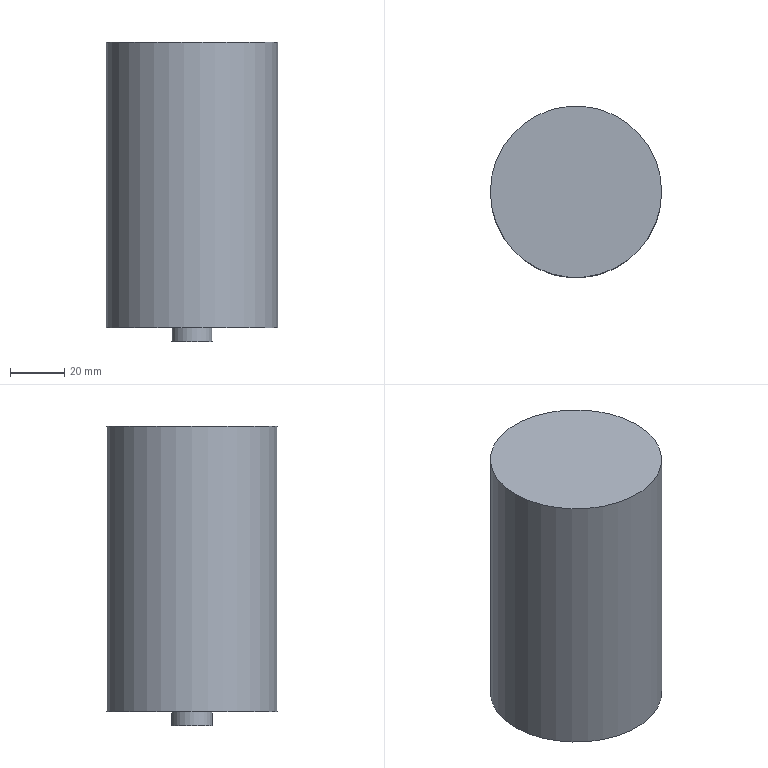Part | NX | features solid 2 | 1 solid | 5 faces | box 63 x 63 x 110 mm | volume 328194 mm3 | plane 3 | cylinder 2 | commonest cylinder face diameters 15 x1 63 x1
STEP:
#1=CARTESIAN_POINT('',(1245.,-607.5,-145.));
#2=VERTEX_POINT('',#1);
#3=CARTESIAN_POINT('',(1245.,-615.,-145.));
#4=DIRECTION('',(0.,0.,1.));
#5=DIRECTION('',(0.,1.,0.));
#6=AXIS2_PLACEMENT_3D('',#3,#4,#5);
#7=CIRCLE('',#6,7.5);
#8=EDGE_CURVE('',#2,#2,#7,.T.);
#9=ORIENTED_EDGE('',*,*,#8,.F.);
#10=EDGE_LOOP('',(#9));
#11=FACE_BOUND('',#10,.T.);
#12=CARTESIAN_POINT('',(1245.,-615.,-145.));
#13=DIRECTION('',(0.,0.,-1.));
#14=DIRECTION('',(0.,-1.,0.));
#15=AXIS2_PLACEMENT_3D('',#12,#13,#14);
#16=PLANE('',#15);
#17=ADVANCED_FACE('',(#11),#16,.T.);
#18=CARTESIAN_POINT('',(1245.,-607.5,-140.));
#19=VERTEX_POINT('',#18);
#20=CARTESIAN_POINT('',(1245.,-615.,-140.));
#21=DIRECTION('',(0.,0.,1.));
#22=DIRECTION('',(0.,1.,0.));
#23=AXIS2_PLACEMENT_3D('',#20,#21,#22);
#24=CIRCLE('',#23,7.5);
#25=EDGE_CURVE('',#19,#19,#24,.T.);
#26=ORIENTED_EDGE('',*,*,#25,.F.);
#27=EDGE_LOOP('',(#26));
#28=FACE_BOUND('',#27,.T.);
#29=ORIENTED_EDGE('',*,*,#8,.T.);
#30=EDGE_LOOP('',(#29));
#31=FACE_BOUND('',#30,.T.);
#32=CARTESIAN_POINT('',(1245.,-615.,-140.));
#33=DIRECTION('',(0.,0.,1.));
#34=DIRECTION('',(0.,1.,0.));
#35=AXIS2_PLACEMENT_3D('',#32,#33,#34);
#36=CYLINDRICAL_SURFACE('',#35,7.5);
#37=ADVANCED_FACE('',(#28,#31),#36,.T.);
#38=CARTESIAN_POINT('',(1213.5,-615.,-35.));
#39=VERTEX_POINT('',#38);
#40=CARTESIAN_POINT('',(1245.,-615.,-35.));
#41=DIRECTION('',(0.,0.,-1.));
#42=DIRECTION('',(-1.,0.,0.));
#43=AXIS2_PLACEMENT_3D('',#40,#41,#42);
#44=CIRCLE('',#43,31.5);
#45=EDGE_CURVE('',#39,#39,#44,.T.);
#46=ORIENTED_EDGE('',*,*,#45,.F.);
#47=EDGE_LOOP('',(#46));
#48=FACE_BOUND('',#47,.T.);
#49=CARTESIAN_POINT('',(1250.,-750.,-35.));
#50=DIRECTION('',(0.,0.,1.));
#51=DIRECTION('',(0.,-1.,0.));
#52=AXIS2_PLACEMENT_3D('',#49,#50,#51);
#53=PLANE('',#52);
#54=ADVANCED_FACE('',(#48),#53,.T.);
#55=ORIENTED_EDGE('',*,*,#25,.T.);
#56=EDGE_LOOP('',(#55));
#57=FACE_BOUND('',#56,.T.);
#58=CARTESIAN_POINT('',(1276.5,-615.,-140.));
#59=VERTEX_POINT('',#58);
#60=CARTESIAN_POINT('',(1245.,-615.,-140.));
#61=DIRECTION('',(0.,0.,1.));
#62=DIRECTION('',(1.,0.,0.));
#63=AXIS2_PLACEMENT_3D('',#60,#61,#62);
#64=CIRCLE('',#63,31.5);
#65=EDGE_CURVE('',#59,#59,#64,.T.);
#66=ORIENTED_EDGE('',*,*,#65,.F.);
#67=EDGE_LOOP('',(#66));
#68=FACE_BOUND('',#67,.T.);
#69=CARTESIAN_POINT('',(1245.,-615.,-140.));
#70=DIRECTION('',(0.,0.,-1.));
#71=DIRECTION('',(0.,-1.,0.));
#72=AXIS2_PLACEMENT_3D('',#69,#70,#71);
#73=PLANE('',#72);
#74=ADVANCED_FACE('',(#57,#68),#73,.T.);
#75=ORIENTED_EDGE('',*,*,#45,.T.);
#76=EDGE_LOOP('',(#75));
#77=FACE_BOUND('',#76,.T.);
#78=ORIENTED_EDGE('',*,*,#65,.T.);
#79=EDGE_LOOP('',(#78));
#80=FACE_BOUND('',#79,.T.);
#81=CARTESIAN_POINT('',(1245.,-615.,-135.));
#82=DIRECTION('',(0.,0.,1.));
#83=DIRECTION('',(0.,1.,0.));
#84=AXIS2_PLACEMENT_3D('',#81,#82,#83);
#85=CYLINDRICAL_SURFACE('',#84,31.5);
#86=ADVANCED_FACE('',(#77,#80),#85,.T.);
#87=CLOSED_SHELL('',(#17,#37,#54,#74,#86));
#88=MANIFOLD_SOLID_BREP('',#87);
#89=(LENGTH_UNIT()NAMED_UNIT(*)SI_UNIT(.MILLI.,.METRE.));
#90=UNCERTAINTY_MEASURE_WITH_UNIT(LENGTH_MEASURE(0.00001),#89,'','');
#91=(NAMED_UNIT(*)PLANE_ANGLE_UNIT()SI_UNIT($,.RADIAN.));
#92=(NAMED_UNIT(*)SI_UNIT($,.STERADIAN.)SOLID_ANGLE_UNIT());
#93=(GEOMETRIC_REPRESENTATION_CONTEXT(3)GLOBAL_UNCERTAINTY_ASSIGNED_CONTEXT((#90))GLOBAL_UNIT_ASSIGNED_CONTEXT((#89,#91,#92))REPRESENTATION_CONTEXT('',''));
#94=ADVANCED_BREP_SHAPE_REPRESENTATION('',(#88),#93);